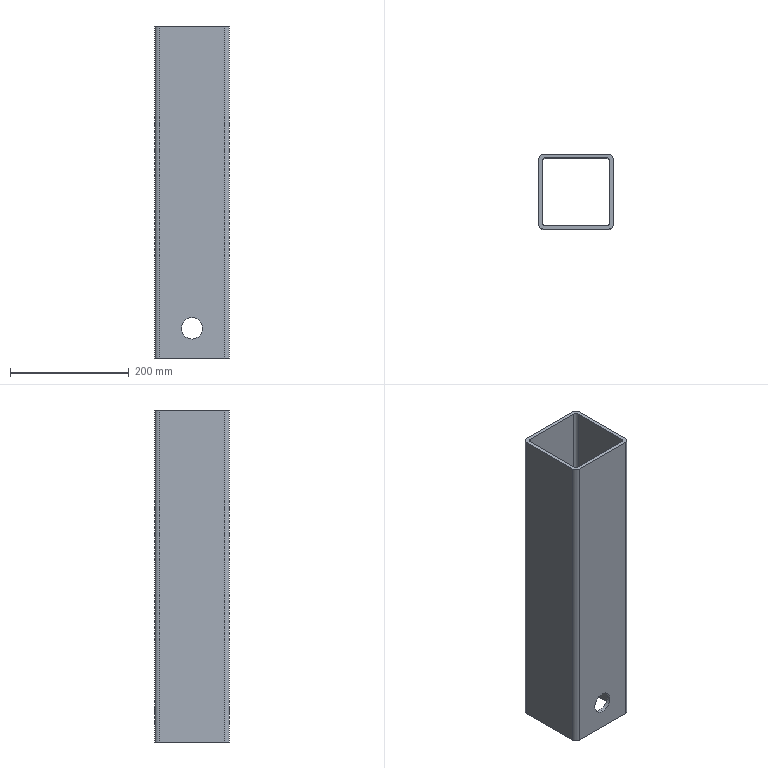Part | SolidWorks | features Fillet 2, Extrusion 1, ICE 1 | 1 solid | 22 faces | box 126 x 126 x 560 mm | volume 1581838 mm3 | cylinder 12 | plane 10 | commonest cylinder face diameters 10 x4 16 x4 36 x4
STEP:
#1=CARTESIAN_POINT('',(63.,6.,32.));
#2=VERTEX_POINT('',#1);
#3=CARTESIAN_POINT('',(63.,6.,68.));
#4=VERTEX_POINT('',#3);
#5=CARTESIAN_POINT('',(63.,6.,50.));
#6=DIRECTION('',(0.,1.,0.));
#7=DIRECTION('',(-1.,0.,0.));
#8=AXIS2_PLACEMENT_3D('',#5,#6,#7);
#9=CIRCLE('',#8,18.);
#10=EDGE_CURVE('',#2,#4,#9,.T.);
#11=ORIENTED_EDGE('',*,*,#10,.T.);
#12=CARTESIAN_POINT('',(63.,0.,68.));
#13=VERTEX_POINT('',#12);
#14=CARTESIAN_POINT('',(63.,260.,68.));
#15=DIRECTION('',(0.,-1.,0.));
#16=VECTOR('',#15,1000.);
#17=LINE('',#14,#16);
#18=EDGE_CURVE('',#4,#13,#17,.T.);
#19=ORIENTED_EDGE('',*,*,#18,.T.);
#20=CARTESIAN_POINT('',(63.,0.,32.));
#21=VERTEX_POINT('',#20);
#22=CARTESIAN_POINT('',(63.,0.,50.));
#23=DIRECTION('',(0.,-1.,0.));
#24=DIRECTION('',(0.,0.,-1.));
#25=AXIS2_PLACEMENT_3D('',#22,#23,#24);
#26=CIRCLE('',#25,18.);
#27=EDGE_CURVE('',#13,#21,#26,.T.);
#28=ORIENTED_EDGE('',*,*,#27,.T.);
#29=CARTESIAN_POINT('',(63.,260.,32.));
#30=DIRECTION('',(0.,-1.,0.));
#31=VECTOR('',#30,1000.);
#32=LINE('',#29,#31);
#33=EDGE_CURVE('',#2,#21,#32,.T.);
#34=ORIENTED_EDGE('',*,*,#33,.F.);
#35=EDGE_LOOP('',(#11,#19,#28,#34));
#36=FACE_OUTER_BOUND('',#35,.T.);
#37=CARTESIAN_POINT('',(63.,260.,50.));
#38=DIRECTION('',(0.,-1.,0.));
#39=DIRECTION('',(0.,0.,-1.));
#40=AXIS2_PLACEMENT_3D('',#37,#38,#39);
#41=CYLINDRICAL_SURFACE('',#40,18.);
#42=ADVANCED_FACE('',(#36),#41,.F.);
#43=CARTESIAN_POINT('',(63.,126.,68.));
#44=VERTEX_POINT('',#43);
#45=CARTESIAN_POINT('',(63.,126.,32.));
#46=VERTEX_POINT('',#45);
#47=CARTESIAN_POINT('',(63.,126.,50.));
#48=DIRECTION('',(0.,-1.,0.));
#49=DIRECTION('',(0.,0.,-1.));
#50=AXIS2_PLACEMENT_3D('',#47,#48,#49);
#51=CIRCLE('',#50,18.);
#52=EDGE_CURVE('',#44,#46,#51,.T.);
#53=ORIENTED_EDGE('',*,*,#52,.F.);
#54=CARTESIAN_POINT('',(63.,120.,68.));
#55=VERTEX_POINT('',#54);
#56=CARTESIAN_POINT('',(63.,260.,68.));
#57=DIRECTION('',(0.,-1.,0.));
#58=VECTOR('',#57,1000.);
#59=LINE('',#56,#58);
#60=EDGE_CURVE('',#44,#55,#59,.T.);
#61=ORIENTED_EDGE('',*,*,#60,.T.);
#62=CARTESIAN_POINT('',(63.,120.,32.));
#63=VERTEX_POINT('',#62);
#64=CARTESIAN_POINT('',(63.,120.,50.));
#65=DIRECTION('',(0.,-1.,0.));
#66=DIRECTION('',(0.,0.,-1.));
#67=AXIS2_PLACEMENT_3D('',#64,#65,#66);
#68=CIRCLE('',#67,18.);
#69=EDGE_CURVE('',#55,#63,#68,.T.);
#70=ORIENTED_EDGE('',*,*,#69,.T.);
#71=CARTESIAN_POINT('',(63.,260.,32.));
#72=DIRECTION('',(0.,-1.,0.));
#73=VECTOR('',#72,1000.);
#74=LINE('',#71,#73);
#75=EDGE_CURVE('',#46,#63,#74,.T.);
#76=ORIENTED_EDGE('',*,*,#75,.F.);
#77=EDGE_LOOP('',(#53,#61,#70,#76));
#78=FACE_OUTER_BOUND('',#77,.T.);
#79=CARTESIAN_POINT('',(63.,260.,50.));
#80=DIRECTION('',(0.,-1.,0.));
#81=DIRECTION('',(0.,0.,-1.));
#82=AXIS2_PLACEMENT_3D('',#79,#80,#81);
#83=CYLINDRICAL_SURFACE('',#82,18.);
#84=ADVANCED_FACE('',(#78),#83,.F.);
#85=CARTESIAN_POINT('',(8.,0.,560.));
#86=VERTEX_POINT('',#85);
#87=CARTESIAN_POINT('',(118.,0.,560.));
#88=VERTEX_POINT('',#87);
#89=CARTESIAN_POINT('',(0.,0.,560.));
#90=DIRECTION('',(1.,0.,0.));
#91=VECTOR('',#90,1000.);
#92=LINE('',#89,#91);
#93=EDGE_CURVE('',#86,#88,#92,.T.);
#94=ORIENTED_EDGE('',*,*,#93,.T.);
#95=CARTESIAN_POINT('',(126.,8.,560.));
#96=VERTEX_POINT('',#95);
#97=CARTESIAN_POINT('',(118.,8.,560.));
#98=DIRECTION('',(0.,0.,1.));
#99=DIRECTION('',(-1.,0.,0.));
#100=AXIS2_PLACEMENT_3D('',#97,#98,#99);
#101=CIRCLE('',#100,8.);
#102=EDGE_CURVE('',#88,#96,#101,.T.);
#103=ORIENTED_EDGE('',*,*,#102,.T.);
#104=CARTESIAN_POINT('',(126.,118.,560.));
#105=VERTEX_POINT('',#104);
#106=CARTESIAN_POINT('',(126.,0.,560.));
#107=DIRECTION('',(0.,1.,0.));
#108=VECTOR('',#107,1000.);
#109=LINE('',#106,#108);
#110=EDGE_CURVE('',#96,#105,#109,.T.);
#111=ORIENTED_EDGE('',*,*,#110,.T.);
#112=CARTESIAN_POINT('',(118.,126.,560.));
#113=VERTEX_POINT('',#112);
#114=CARTESIAN_POINT('',(118.,118.,560.));
#115=DIRECTION('',(0.,0.,1.));
#116=DIRECTION('',(-1.,0.,0.));
#117=AXIS2_PLACEMENT_3D('',#114,#115,#116);
#118=CIRCLE('',#117,8.);
#119=EDGE_CURVE('',#105,#113,#118,.T.);
#120=ORIENTED_EDGE('',*,*,#119,.T.);
#121=CARTESIAN_POINT('',(8.,126.,560.));
#122=VERTEX_POINT('',#121);
#123=CARTESIAN_POINT('',(0.,126.,560.));
#124=DIRECTION('',(-1.,0.,0.));
#125=VECTOR('',#124,1000.);
#126=LINE('',#123,#125);
#127=EDGE_CURVE('',#113,#122,#126,.T.);
#128=ORIENTED_EDGE('',*,*,#127,.T.);
#129=CARTESIAN_POINT('',(0.,118.,560.));
#130=VERTEX_POINT('',#129);
#131=CARTESIAN_POINT('',(8.,118.,560.));
#132=DIRECTION('',(0.,0.,1.));
#133=DIRECTION('',(-1.,0.,0.));
#134=AXIS2_PLACEMENT_3D('',#131,#132,#133);
#135=CIRCLE('',#134,8.);
#136=EDGE_CURVE('',#122,#130,#135,.T.);
#137=ORIENTED_EDGE('',*,*,#136,.T.);
#138=CARTESIAN_POINT('',(0.,8.,560.));
#139=VERTEX_POINT('',#138);
#140=CARTESIAN_POINT('',(0.,0.,560.));
#141=DIRECTION('',(0.,-1.,0.));
#142=VECTOR('',#141,1000.);
#143=LINE('',#140,#142);
#144=EDGE_CURVE('',#130,#139,#143,.T.);
#145=ORIENTED_EDGE('',*,*,#144,.T.);
#146=CARTESIAN_POINT('',(8.,8.,560.));
#147=DIRECTION('',(0.,0.,1.));
#148=DIRECTION('',(-1.,0.,0.));
#149=AXIS2_PLACEMENT_3D('',#146,#147,#148);
#150=CIRCLE('',#149,8.);
#151=EDGE_CURVE('',#139,#86,#150,.T.);
#152=ORIENTED_EDGE('',*,*,#151,.T.);
#153=EDGE_LOOP('',(#94,#103,#111,#120,#128,#137,#145,#152));
#154=FACE_OUTER_BOUND('',#153,.T.);
#155=CARTESIAN_POINT('',(6.,115.,560.));
#156=VERTEX_POINT('',#155);
#157=CARTESIAN_POINT('',(6.,11.,560.));
#158=VERTEX_POINT('',#157);
#159=CARTESIAN_POINT('',(6.,120.,560.));
#160=DIRECTION('',(0.,-1.,0.));
#161=VECTOR('',#160,1000.);
#162=LINE('',#159,#161);
#163=EDGE_CURVE('',#156,#158,#162,.T.);
#164=ORIENTED_EDGE('',*,*,#163,.F.);
#165=CARTESIAN_POINT('',(11.,120.,560.));
#166=VERTEX_POINT('',#165);
#167=CARTESIAN_POINT('',(11.,115.,560.));
#168=DIRECTION('',(0.,0.,-1.));
#169=DIRECTION('',(-1.,0.,0.));
#170=AXIS2_PLACEMENT_3D('',#167,#168,#169);
#171=CIRCLE('',#170,5.);
#172=EDGE_CURVE('',#156,#166,#171,.T.);
#173=ORIENTED_EDGE('',*,*,#172,.T.);
#174=CARTESIAN_POINT('',(115.,120.,560.));
#175=VERTEX_POINT('',#174);
#176=CARTESIAN_POINT('',(6.,120.,560.));
#177=DIRECTION('',(-1.,0.,0.));
#178=VECTOR('',#177,1000.);
#179=LINE('',#176,#178);
#180=EDGE_CURVE('',#175,#166,#179,.T.);
#181=ORIENTED_EDGE('',*,*,#180,.F.);
#182=CARTESIAN_POINT('',(120.,115.,560.));
#183=VERTEX_POINT('',#182);
#184=CARTESIAN_POINT('',(115.,115.,560.));
#185=DIRECTION('',(0.,0.,-1.));
#186=DIRECTION('',(-1.,0.,0.));
#187=AXIS2_PLACEMENT_3D('',#184,#185,#186);
#188=CIRCLE('',#187,5.);
#189=EDGE_CURVE('',#175,#183,#188,.T.);
#190=ORIENTED_EDGE('',*,*,#189,.T.);
#191=CARTESIAN_POINT('',(120.,11.,560.));
#192=VERTEX_POINT('',#191);
#193=CARTESIAN_POINT('',(120.,120.,560.));
#194=DIRECTION('',(0.,1.,0.));
#195=VECTOR('',#194,1000.);
#196=LINE('',#193,#195);
#197=EDGE_CURVE('',#192,#183,#196,.T.);
#198=ORIENTED_EDGE('',*,*,#197,.F.);
#199=CARTESIAN_POINT('',(115.,6.,560.));
#200=VERTEX_POINT('',#199);
#201=CARTESIAN_POINT('',(115.,11.,560.));
#202=DIRECTION('',(0.,0.,-1.));
#203=DIRECTION('',(-1.,0.,0.));
#204=AXIS2_PLACEMENT_3D('',#201,#202,#203);
#205=CIRCLE('',#204,5.);
#206=EDGE_CURVE('',#192,#200,#205,.T.);
#207=ORIENTED_EDGE('',*,*,#206,.T.);
#208=CARTESIAN_POINT('',(11.,6.,560.));
#209=VERTEX_POINT('',#208);
#210=CARTESIAN_POINT('',(6.,6.,560.));
#211=DIRECTION('',(1.,0.,0.));
#212=VECTOR('',#211,1000.);
#213=LINE('',#210,#212);
#214=EDGE_CURVE('',#209,#200,#213,.T.);
#215=ORIENTED_EDGE('',*,*,#214,.F.);
#216=CARTESIAN_POINT('',(11.,11.,560.));
#217=DIRECTION('',(0.,0.,-1.));
#218=DIRECTION('',(-1.,0.,0.));
#219=AXIS2_PLACEMENT_3D('',#216,#217,#218);
#220=CIRCLE('',#219,5.);
#221=EDGE_CURVE('',#209,#158,#220,.T.);
#222=ORIENTED_EDGE('',*,*,#221,.T.);
#223=EDGE_LOOP('',(#164,#173,#181,#190,#198,#207,#215,#222));
#224=FACE_BOUND('',#223,.T.);
#225=CARTESIAN_POINT('',(0.,0.,560.));
#226=DIRECTION('',(0.,0.,-1.));
#227=DIRECTION('',(-1.,0.,0.));
#228=AXIS2_PLACEMENT_3D('',#225,#226,#227);
#229=PLANE('',#228);
#230=ADVANCED_FACE('',(#154,#224),#229,.F.);
#231=CARTESIAN_POINT('',(126.,8.,0.));
#232=VERTEX_POINT('',#231);
#233=CARTESIAN_POINT('',(126.,118.,0.));
#234=VERTEX_POINT('',#233);
#235=CARTESIAN_POINT('',(126.,0.,0.));
#236=DIRECTION('',(0.,1.,0.));
#237=VECTOR('',#236,1000.);
#238=LINE('',#235,#237);
#239=EDGE_CURVE('',#232,#234,#238,.T.);
#240=ORIENTED_EDGE('',*,*,#239,.F.);
#241=CARTESIAN_POINT('',(118.,0.,0.));
#242=VERTEX_POINT('',#241);
#243=CARTESIAN_POINT('',(118.,8.,0.));
#244=DIRECTION('',(0.,0.,-1.));
#245=DIRECTION('',(-1.,0.,0.));
#246=AXIS2_PLACEMENT_3D('',#243,#244,#245);
#247=CIRCLE('',#246,8.);
#248=EDGE_CURVE('',#232,#242,#247,.T.);
#249=ORIENTED_EDGE('',*,*,#248,.T.);
#250=CARTESIAN_POINT('',(8.,0.,0.));
#251=VERTEX_POINT('',#250);
#252=CARTESIAN_POINT('',(0.,0.,0.));
#253=DIRECTION('',(1.,0.,0.));
#254=VECTOR('',#253,1000.);
#255=LINE('',#252,#254);
#256=EDGE_CURVE('',#251,#242,#255,.T.);
#257=ORIENTED_EDGE('',*,*,#256,.F.);
#258=CARTESIAN_POINT('',(0.,8.,0.));
#259=VERTEX_POINT('',#258);
#260=CARTESIAN_POINT('',(8.,8.,0.));
#261=DIRECTION('',(0.,0.,-1.));
#262=DIRECTION('',(-1.,0.,0.));
#263=AXIS2_PLACEMENT_3D('',#260,#261,#262);
#264=CIRCLE('',#263,8.);
#265=EDGE_CURVE('',#251,#259,#264,.T.);
#266=ORIENTED_EDGE('',*,*,#265,.T.);
#267=CARTESIAN_POINT('',(0.,118.,0.));
#268=VERTEX_POINT('',#267);
#269=CARTESIAN_POINT('',(0.,0.,0.));
#270=DIRECTION('',(0.,-1.,0.));
#271=VECTOR('',#270,1000.);
#272=LINE('',#269,#271);
#273=EDGE_CURVE('',#268,#259,#272,.T.);
#274=ORIENTED_EDGE('',*,*,#273,.F.);
#275=CARTESIAN_POINT('',(8.,126.,0.));
#276=VERTEX_POINT('',#275);
#277=CARTESIAN_POINT('',(8.,118.,0.));
#278=DIRECTION('',(0.,0.,-1.));
#279=DIRECTION('',(-1.,0.,0.));
#280=AXIS2_PLACEMENT_3D('',#277,#278,#279);
#281=CIRCLE('',#280,8.);
#282=EDGE_CURVE('',#268,#276,#281,.T.);
#283=ORIENTED_EDGE('',*,*,#282,.T.);
#284=CARTESIAN_POINT('',(118.,126.,0.));
#285=VERTEX_POINT('',#284);
#286=CARTESIAN_POINT('',(0.,126.,0.));
#287=DIRECTION('',(-1.,0.,0.));
#288=VECTOR('',#287,1000.);
#289=LINE('',#286,#288);
#290=EDGE_CURVE('',#285,#276,#289,.T.);
#291=ORIENTED_EDGE('',*,*,#290,.F.);
#292=CARTESIAN_POINT('',(118.,118.,0.));
#293=DIRECTION('',(0.,0.,-1.));
#294=DIRECTION('',(-1.,0.,0.));
#295=AXIS2_PLACEMENT_3D('',#292,#293,#294);
#296=CIRCLE('',#295,8.);
#297=EDGE_CURVE('',#285,#234,#296,.T.);
#298=ORIENTED_EDGE('',*,*,#297,.T.);
#299=EDGE_LOOP('',(#240,#249,#257,#266,#274,#283,#291,#298));
#300=FACE_OUTER_BOUND('',#299,.T.);
#301=CARTESIAN_POINT('',(120.,11.,0.));
#302=VERTEX_POINT('',#301);
#303=CARTESIAN_POINT('',(120.,115.,0.));
#304=VERTEX_POINT('',#303);
#305=CARTESIAN_POINT('',(120.,120.,0.));
#306=DIRECTION('',(0.,1.,0.));
#307=VECTOR('',#306,1000.);
#308=LINE('',#305,#307);
#309=EDGE_CURVE('',#302,#304,#308,.T.);
#310=ORIENTED_EDGE('',*,*,#309,.T.);
#311=CARTESIAN_POINT('',(115.,120.,0.));
#312=VERTEX_POINT('',#311);
#313=CARTESIAN_POINT('',(115.,115.,0.));
#314=DIRECTION('',(0.,0.,1.));
#315=DIRECTION('',(-1.,0.,0.));
#316=AXIS2_PLACEMENT_3D('',#313,#314,#315);
#317=CIRCLE('',#316,5.);
#318=EDGE_CURVE('',#304,#312,#317,.T.);
#319=ORIENTED_EDGE('',*,*,#318,.T.);
#320=CARTESIAN_POINT('',(11.,120.,0.));
#321=VERTEX_POINT('',#320);
#322=CARTESIAN_POINT('',(6.,120.,0.));
#323=DIRECTION('',(-1.,0.,0.));
#324=VECTOR('',#323,1000.);
#325=LINE('',#322,#324);
#326=EDGE_CURVE('',#312,#321,#325,.T.);
#327=ORIENTED_EDGE('',*,*,#326,.T.);
#328=CARTESIAN_POINT('',(6.,115.,0.));
#329=VERTEX_POINT('',#328);
#330=CARTESIAN_POINT('',(11.,115.,0.));
#331=DIRECTION('',(0.,0.,1.));
#332=DIRECTION('',(-1.,0.,0.));
#333=AXIS2_PLACEMENT_3D('',#330,#331,#332);
#334=CIRCLE('',#333,5.);
#335=EDGE_CURVE('',#321,#329,#334,.T.);
#336=ORIENTED_EDGE('',*,*,#335,.T.);
#337=CARTESIAN_POINT('',(6.,11.,0.));
#338=VERTEX_POINT('',#337);
#339=CARTESIAN_POINT('',(6.,120.,0.));
#340=DIRECTION('',(0.,-1.,0.));
#341=VECTOR('',#340,1000.);
#342=LINE('',#339,#341);
#343=EDGE_CURVE('',#329,#338,#342,.T.);
#344=ORIENTED_EDGE('',*,*,#343,.T.);
#345=CARTESIAN_POINT('',(11.,6.,0.));
#346=VERTEX_POINT('',#345);
#347=CARTESIAN_POINT('',(11.,11.,0.));
#348=DIRECTION('',(0.,0.,1.));
#349=DIRECTION('',(-1.,0.,0.));
#350=AXIS2_PLACEMENT_3D('',#347,#348,#349);
#351=CIRCLE('',#350,5.);
#352=EDGE_CURVE('',#338,#346,#351,.T.);
#353=ORIENTED_EDGE('',*,*,#352,.T.);
#354=CARTESIAN_POINT('',(115.,6.,0.));
#355=VERTEX_POINT('',#354);
#356=CARTESIAN_POINT('',(6.,6.,0.));
#357=DIRECTION('',(1.,0.,0.));
#358=VECTOR('',#357,1000.);
#359=LINE('',#356,#358);
#360=EDGE_CURVE('',#346,#355,#359,.T.);
#361=ORIENTED_EDGE('',*,*,#360,.T.);
#362=CARTESIAN_POINT('',(115.,11.,0.));
#363=DIRECTION('',(0.,0.,1.));
#364=DIRECTION('',(-1.,0.,0.));
#365=AXIS2_PLACEMENT_3D('',#362,#363,#364);
#366=CIRCLE('',#365,5.);
#367=EDGE_CURVE('',#355,#302,#366,.T.);
#368=ORIENTED_EDGE('',*,*,#367,.T.);
#369=EDGE_LOOP('',(#310,#319,#327,#336,#344,#353,#361,#368));
#370=FACE_BOUND('',#369,.T.);
#371=CARTESIAN_POINT('',(0.,0.,0.));
#372=DIRECTION('',(0.,0.,-1.));
#373=DIRECTION('',(-1.,0.,0.));
#374=AXIS2_PLACEMENT_3D('',#371,#372,#373);
#375=PLANE('',#374);
#376=ADVANCED_FACE('',(#300,#370),#375,.T.);
#377=ORIENTED_EDGE('',*,*,#273,.T.);
#378=CARTESIAN_POINT('',(0.,8.,560.));
#379=DIRECTION('',(0.,0.,1.));
#380=VECTOR('',#379,1000.);
#381=LINE('',#378,#380);
#382=EDGE_CURVE('',#259,#139,#381,.T.);
#383=ORIENTED_EDGE('',*,*,#382,.T.);
#384=ORIENTED_EDGE('',*,*,#144,.F.);
#385=CARTESIAN_POINT('',(0.,118.,560.));
#386=DIRECTION('',(0.,0.,-1.));
#387=VECTOR('',#386,1000.);
#388=LINE('',#385,#387);
#389=EDGE_CURVE('',#130,#268,#388,.T.);
#390=ORIENTED_EDGE('',*,*,#389,.T.);
#391=EDGE_LOOP('',(#377,#383,#384,#390));
#392=FACE_OUTER_BOUND('',#391,.T.);
#393=CARTESIAN_POINT('',(0.,0.,560.));
#394=DIRECTION('',(1.,0.,0.));
#395=DIRECTION('',(0.,0.,-1.));
#396=AXIS2_PLACEMENT_3D('',#393,#394,#395);
#397=PLANE('',#396);
#398=ADVANCED_FACE('',(#392),#397,.F.);
#399=CARTESIAN_POINT('',(63.,0.,50.));
#400=DIRECTION('',(0.,-1.,0.));
#401=DIRECTION('',(0.,0.,-1.));
#402=AXIS2_PLACEMENT_3D('',#399,#400,#401);
#403=CIRCLE('',#402,18.);
#404=EDGE_CURVE('',#21,#13,#403,.T.);
#405=ORIENTED_EDGE('',*,*,#404,.F.);
#406=ORIENTED_EDGE('',*,*,#27,.F.);
#407=EDGE_LOOP('',(#405,#406));
#408=FACE_BOUND('',#407,.T.);
#409=ORIENTED_EDGE('',*,*,#256,.T.);
#410=CARTESIAN_POINT('',(118.,0.,560.));
#411=DIRECTION('',(0.,0.,1.));
#412=VECTOR('',#411,1000.);
#413=LINE('',#410,#412);
#414=EDGE_CURVE('',#242,#88,#413,.T.);
#415=ORIENTED_EDGE('',*,*,#414,.T.);
#416=ORIENTED_EDGE('',*,*,#93,.F.);
#417=CARTESIAN_POINT('',(8.,0.,560.));
#418=DIRECTION('',(0.,0.,-1.));
#419=VECTOR('',#418,1000.);
#420=LINE('',#417,#419);
#421=EDGE_CURVE('',#86,#251,#420,.T.);
#422=ORIENTED_EDGE('',*,*,#421,.T.);
#423=EDGE_LOOP('',(#409,#415,#416,#422));
#424=FACE_OUTER_BOUND('',#423,.T.);
#425=CARTESIAN_POINT('',(0.,0.,560.));
#426=DIRECTION('',(0.,1.,0.));
#427=DIRECTION('',(0.,0.,1.));
#428=AXIS2_PLACEMENT_3D('',#425,#426,#427);
#429=PLANE('',#428);
#430=ADVANCED_FACE('',(#408,#424),#429,.F.);
#431=ORIENTED_EDGE('',*,*,#110,.F.);
#432=CARTESIAN_POINT('',(126.,8.,560.));
#433=DIRECTION('',(0.,0.,-1.));
#434=VECTOR('',#433,1000.);
#435=LINE('',#432,#434);
#436=EDGE_CURVE('',#96,#232,#435,.T.);
#437=ORIENTED_EDGE('',*,*,#436,.T.);
#438=ORIENTED_EDGE('',*,*,#239,.T.);
#439=CARTESIAN_POINT('',(126.,118.,560.));
#440=DIRECTION('',(0.,0.,1.));
#441=VECTOR('',#440,1000.);
#442=LINE('',#439,#441);
#443=EDGE_CURVE('',#234,#105,#442,.T.);
#444=ORIENTED_EDGE('',*,*,#443,.T.);
#445=EDGE_LOOP('',(#431,#437,#438,#444));
#446=FACE_OUTER_BOUND('',#445,.T.);
#447=CARTESIAN_POINT('',(126.,0.,560.));
#448=DIRECTION('',(-1.,0.,0.));
#449=DIRECTION('',(0.,0.,1.));
#450=AXIS2_PLACEMENT_3D('',#447,#448,#449);
#451=PLANE('',#450);
#452=ADVANCED_FACE('',(#446),#451,.F.);
#453=CARTESIAN_POINT('',(63.,126.,50.));
#454=DIRECTION('',(0.,-1.,0.));
#455=DIRECTION('',(0.,0.,-1.));
#456=AXIS2_PLACEMENT_3D('',#453,#454,#455);
#457=CIRCLE('',#456,18.);
#458=EDGE_CURVE('',#46,#44,#457,.T.);
#459=ORIENTED_EDGE('',*,*,#458,.T.);
#460=ORIENTED_EDGE('',*,*,#52,.T.);
#461=EDGE_LOOP('',(#459,#460));
#462=FACE_BOUND('',#461,.T.);
#463=ORIENTED_EDGE('',*,*,#290,.T.);
#464=CARTESIAN_POINT('',(8.,126.,560.));
#465=DIRECTION('',(0.,0.,1.));
#466=VECTOR('',#465,1000.);
#467=LINE('',#464,#466);
#468=EDGE_CURVE('',#276,#122,#467,.T.);
#469=ORIENTED_EDGE('',*,*,#468,.T.);
#470=ORIENTED_EDGE('',*,*,#127,.F.);
#471=CARTESIAN_POINT('',(118.,126.,560.));
#472=DIRECTION('',(0.,0.,-1.));
#473=VECTOR('',#472,1000.);
#474=LINE('',#471,#473);
#475=EDGE_CURVE('',#113,#285,#474,.T.);
#476=ORIENTED_EDGE('',*,*,#475,.T.);
#477=EDGE_LOOP('',(#463,#469,#470,#476));
#478=FACE_OUTER_BOUND('',#477,.T.);
#479=CARTESIAN_POINT('',(0.,126.,560.));
#480=DIRECTION('',(0.,-1.,0.));
#481=DIRECTION('',(0.,0.,-1.));
#482=AXIS2_PLACEMENT_3D('',#479,#480,#481);
#483=PLANE('',#482);
#484=ADVANCED_FACE('',(#462,#478),#483,.F.);
#485=ORIENTED_EDGE('',*,*,#163,.T.);
#486=CARTESIAN_POINT('',(6.,11.,0.));
#487=DIRECTION('',(0.,0.,-1.));
#488=VECTOR('',#487,1000.);
#489=LINE('',#486,#488);
#490=EDGE_CURVE('',#158,#338,#489,.T.);
#491=ORIENTED_EDGE('',*,*,#490,.T.);
#492=ORIENTED_EDGE('',*,*,#343,.F.);
#493=CARTESIAN_POINT('',(6.,115.,560.));
#494=DIRECTION('',(0.,0.,1.));
#495=VECTOR('',#494,1000.);
#496=LINE('',#493,#495);
#497=EDGE_CURVE('',#329,#156,#496,.T.);
#498=ORIENTED_EDGE('',*,*,#497,.T.);
#499=EDGE_LOOP('',(#485,#491,#492,#498));
#500=FACE_OUTER_BOUND('',#499,.T.);
#501=CARTESIAN_POINT('',(6.,120.,560.));
#502=DIRECTION('',(1.,0.,0.));
#503=DIRECTION('',(0.,1.,0.));
#504=AXIS2_PLACEMENT_3D('',#501,#502,#503);
#505=PLANE('',#504);
#506=ADVANCED_FACE('',(#500),#505,.T.);
#507=ORIENTED_EDGE('',*,*,#10,.F.);
#508=CARTESIAN_POINT('',(63.,6.,50.));
#509=DIRECTION('',(0.,1.,0.));
#510=DIRECTION('',(-1.,0.,0.));
#511=AXIS2_PLACEMENT_3D('',#508,#509,#510);
#512=CIRCLE('',#511,18.);
#513=EDGE_CURVE('',#4,#2,#512,.T.);
#514=ORIENTED_EDGE('',*,*,#513,.F.);
#515=EDGE_LOOP('',(#507,#514));
#516=FACE_BOUND('',#515,.T.);
#517=ORIENTED_EDGE('',*,*,#360,.F.);
#518=CARTESIAN_POINT('',(11.,6.,560.));
#519=DIRECTION('',(0.,0.,1.));
#520=VECTOR('',#519,1000.);
#521=LINE('',#518,#520);
#522=EDGE_CURVE('',#346,#209,#521,.T.);
#523=ORIENTED_EDGE('',*,*,#522,.T.);
#524=ORIENTED_EDGE('',*,*,#214,.T.);
#525=CARTESIAN_POINT('',(115.,6.,0.));
#526=DIRECTION('',(0.,0.,-1.));
#527=VECTOR('',#526,1000.);
#528=LINE('',#525,#527);
#529=EDGE_CURVE('',#200,#355,#528,.T.);
#530=ORIENTED_EDGE('',*,*,#529,.T.);
#531=EDGE_LOOP('',(#517,#523,#524,#530));
#532=FACE_OUTER_BOUND('',#531,.T.);
#533=CARTESIAN_POINT('',(6.,6.,560.));
#534=DIRECTION('',(0.,1.,0.));
#535=DIRECTION('',(-1.,0.,0.));
#536=AXIS2_PLACEMENT_3D('',#533,#534,#535);
#537=PLANE('',#536);
#538=ADVANCED_FACE('',(#516,#532),#537,.T.);
#539=ORIENTED_EDGE('',*,*,#309,.F.);
#540=CARTESIAN_POINT('',(120.,11.,560.));
#541=DIRECTION('',(0.,0.,1.));
#542=VECTOR('',#541,1000.);
#543=LINE('',#540,#542);
#544=EDGE_CURVE('',#302,#192,#543,.T.);
#545=ORIENTED_EDGE('',*,*,#544,.T.);
#546=ORIENTED_EDGE('',*,*,#197,.T.);
#547=CARTESIAN_POINT('',(120.,115.,0.));
#548=DIRECTION('',(0.,0.,-1.));
#549=VECTOR('',#548,1000.);
#550=LINE('',#547,#549);
#551=EDGE_CURVE('',#183,#304,#550,.T.);
#552=ORIENTED_EDGE('',*,*,#551,.T.);
#553=EDGE_LOOP('',(#539,#545,#546,#552));
#554=FACE_OUTER_BOUND('',#553,.T.);
#555=CARTESIAN_POINT('',(120.,120.,560.));
#556=DIRECTION('',(-1.,0.,0.));
#557=DIRECTION('',(0.,-1.,0.));
#558=AXIS2_PLACEMENT_3D('',#555,#556,#557);
#559=PLANE('',#558);
#560=ADVANCED_FACE('',(#554),#559,.T.);
#561=CARTESIAN_POINT('',(63.,120.,50.));
#562=DIRECTION('',(0.,-1.,0.));
#563=DIRECTION('',(0.,0.,-1.));
#564=AXIS2_PLACEMENT_3D('',#561,#562,#563);
#565=CIRCLE('',#564,18.);
#566=EDGE_CURVE('',#63,#55,#565,.T.);
#567=ORIENTED_EDGE('',*,*,#566,.F.);
#568=ORIENTED_EDGE('',*,*,#69,.F.);
#569=EDGE_LOOP('',(#567,#568));
#570=FACE_BOUND('',#569,.T.);
#571=ORIENTED_EDGE('',*,*,#326,.F.);
#572=CARTESIAN_POINT('',(115.,120.,560.));
#573=DIRECTION('',(0.,0.,1.));
#574=VECTOR('',#573,1000.);
#575=LINE('',#572,#574);
#576=EDGE_CURVE('',#312,#175,#575,.T.);
#577=ORIENTED_EDGE('',*,*,#576,.T.);
#578=ORIENTED_EDGE('',*,*,#180,.T.);
#579=CARTESIAN_POINT('',(11.,120.,0.));
#580=DIRECTION('',(0.,0.,-1.));
#581=VECTOR('',#580,1000.);
#582=LINE('',#579,#581);
#583=EDGE_CURVE('',#166,#321,#582,.T.);
#584=ORIENTED_EDGE('',*,*,#583,.T.);
#585=EDGE_LOOP('',(#571,#577,#578,#584));
#586=FACE_OUTER_BOUND('',#585,.T.);
#587=CARTESIAN_POINT('',(6.,120.,560.));
#588=DIRECTION('',(0.,-1.,0.));
#589=DIRECTION('',(0.,0.,-1.));
#590=AXIS2_PLACEMENT_3D('',#587,#588,#589);
#591=PLANE('',#590);
#592=ADVANCED_FACE('',(#570,#586),#591,.T.);
#593=ORIENTED_EDGE('',*,*,#102,.F.);
#594=ORIENTED_EDGE('',*,*,#414,.F.);
#595=ORIENTED_EDGE('',*,*,#248,.F.);
#596=ORIENTED_EDGE('',*,*,#436,.F.);
#597=EDGE_LOOP('',(#593,#594,#595,#596));
#598=FACE_OUTER_BOUND('',#597,.T.);
#599=CARTESIAN_POINT('',(118.,8.,560.));
#600=DIRECTION('',(0.,0.,-1.));
#601=DIRECTION('',(-1.,0.,0.));
#602=AXIS2_PLACEMENT_3D('',#599,#600,#601);
#603=CYLINDRICAL_SURFACE('',#602,8.);
#604=ADVANCED_FACE('',(#598),#603,.T.);
#605=ORIENTED_EDGE('',*,*,#151,.F.);
#606=ORIENTED_EDGE('',*,*,#382,.F.);
#607=ORIENTED_EDGE('',*,*,#265,.F.);
#608=ORIENTED_EDGE('',*,*,#421,.F.);
#609=EDGE_LOOP('',(#605,#606,#607,#608));
#610=FACE_OUTER_BOUND('',#609,.T.);
#611=CARTESIAN_POINT('',(8.,8.,560.));
#612=DIRECTION('',(0.,0.,-1.));
#613=DIRECTION('',(-1.,0.,0.));
#614=AXIS2_PLACEMENT_3D('',#611,#612,#613);
#615=CYLINDRICAL_SURFACE('',#614,8.);
#616=ADVANCED_FACE('',(#610),#615,.T.);
#617=ORIENTED_EDGE('',*,*,#136,.F.);
#618=ORIENTED_EDGE('',*,*,#468,.F.);
#619=ORIENTED_EDGE('',*,*,#282,.F.);
#620=ORIENTED_EDGE('',*,*,#389,.F.);
#621=EDGE_LOOP('',(#617,#618,#619,#620));
#622=FACE_OUTER_BOUND('',#621,.T.);
#623=CARTESIAN_POINT('',(8.,118.,560.));
#624=DIRECTION('',(0.,0.,-1.));
#625=DIRECTION('',(-1.,0.,0.));
#626=AXIS2_PLACEMENT_3D('',#623,#624,#625);
#627=CYLINDRICAL_SURFACE('',#626,8.);
#628=ADVANCED_FACE('',(#622),#627,.T.);
#629=ORIENTED_EDGE('',*,*,#119,.F.);
#630=ORIENTED_EDGE('',*,*,#443,.F.);
#631=ORIENTED_EDGE('',*,*,#297,.F.);
#632=ORIENTED_EDGE('',*,*,#475,.F.);
#633=EDGE_LOOP('',(#629,#630,#631,#632));
#634=FACE_OUTER_BOUND('',#633,.T.);
#635=CARTESIAN_POINT('',(118.,118.,560.));
#636=DIRECTION('',(0.,0.,-1.));
#637=DIRECTION('',(-1.,0.,0.));
#638=AXIS2_PLACEMENT_3D('',#635,#636,#637);
#639=CYLINDRICAL_SURFACE('',#638,8.);
#640=ADVANCED_FACE('',(#634),#639,.T.);
#641=ORIENTED_EDGE('',*,*,#221,.F.);
#642=ORIENTED_EDGE('',*,*,#522,.F.);
#643=ORIENTED_EDGE('',*,*,#352,.F.);
#644=ORIENTED_EDGE('',*,*,#490,.F.);
#645=EDGE_LOOP('',(#641,#642,#643,#644));
#646=FACE_OUTER_BOUND('',#645,.T.);
#647=CARTESIAN_POINT('',(11.,11.,560.));
#648=DIRECTION('',(0.,0.,1.));
#649=DIRECTION('',(1.,0.,0.));
#650=AXIS2_PLACEMENT_3D('',#647,#648,#649);
#651=CYLINDRICAL_SURFACE('',#650,5.);
#652=ADVANCED_FACE('',(#646),#651,.F.);
#653=ORIENTED_EDGE('',*,*,#206,.F.);
#654=ORIENTED_EDGE('',*,*,#544,.F.);
#655=ORIENTED_EDGE('',*,*,#367,.F.);
#656=ORIENTED_EDGE('',*,*,#529,.F.);
#657=EDGE_LOOP('',(#653,#654,#655,#656));
#658=FACE_OUTER_BOUND('',#657,.T.);
#659=CARTESIAN_POINT('',(115.,11.,560.));
#660=DIRECTION('',(0.,0.,1.));
#661=DIRECTION('',(1.,0.,0.));
#662=AXIS2_PLACEMENT_3D('',#659,#660,#661);
#663=CYLINDRICAL_SURFACE('',#662,5.);
#664=ADVANCED_FACE('',(#658),#663,.F.);
#665=ORIENTED_EDGE('',*,*,#189,.F.);
#666=ORIENTED_EDGE('',*,*,#576,.F.);
#667=ORIENTED_EDGE('',*,*,#318,.F.);
#668=ORIENTED_EDGE('',*,*,#551,.F.);
#669=EDGE_LOOP('',(#665,#666,#667,#668));
#670=FACE_OUTER_BOUND('',#669,.T.);
#671=CARTESIAN_POINT('',(115.,115.,560.));
#672=DIRECTION('',(0.,0.,1.));
#673=DIRECTION('',(1.,0.,0.));
#674=AXIS2_PLACEMENT_3D('',#671,#672,#673);
#675=CYLINDRICAL_SURFACE('',#674,5.);
#676=ADVANCED_FACE('',(#670),#675,.F.);
#677=ORIENTED_EDGE('',*,*,#172,.F.);
#678=ORIENTED_EDGE('',*,*,#497,.F.);
#679=ORIENTED_EDGE('',*,*,#335,.F.);
#680=ORIENTED_EDGE('',*,*,#583,.F.);
#681=EDGE_LOOP('',(#677,#678,#679,#680));
#682=FACE_OUTER_BOUND('',#681,.T.);
#683=CARTESIAN_POINT('',(11.,115.,560.));
#684=DIRECTION('',(0.,0.,1.));
#685=DIRECTION('',(1.,0.,0.));
#686=AXIS2_PLACEMENT_3D('',#683,#684,#685);
#687=CYLINDRICAL_SURFACE('',#686,5.);
#688=ADVANCED_FACE('',(#682),#687,.F.);
#689=ORIENTED_EDGE('',*,*,#60,.F.);
#690=ORIENTED_EDGE('',*,*,#458,.F.);
#691=ORIENTED_EDGE('',*,*,#75,.T.);
#692=ORIENTED_EDGE('',*,*,#566,.T.);
#693=EDGE_LOOP('',(#689,#690,#691,#692));
#694=FACE_OUTER_BOUND('',#693,.T.);
#695=CARTESIAN_POINT('',(63.,260.,50.));
#696=DIRECTION('',(0.,-1.,0.));
#697=DIRECTION('',(0.,0.,-1.));
#698=AXIS2_PLACEMENT_3D('',#695,#696,#697);
#699=CYLINDRICAL_SURFACE('',#698,18.);
#700=ADVANCED_FACE('',(#694),#699,.F.);
#701=ORIENTED_EDGE('',*,*,#18,.F.);
#702=ORIENTED_EDGE('',*,*,#513,.T.);
#703=ORIENTED_EDGE('',*,*,#33,.T.);
#704=ORIENTED_EDGE('',*,*,#404,.T.);
#705=EDGE_LOOP('',(#701,#702,#703,#704));
#706=FACE_OUTER_BOUND('',#705,.T.);
#707=CARTESIAN_POINT('',(63.,260.,50.));
#708=DIRECTION('',(0.,-1.,0.));
#709=DIRECTION('',(0.,0.,-1.));
#710=AXIS2_PLACEMENT_3D('',#707,#708,#709);
#711=CYLINDRICAL_SURFACE('',#710,18.);
#712=ADVANCED_FACE('',(#706),#711,.F.);
#713=CLOSED_SHELL('',(#42,#84,#230,#376,#398,#430,#452,#484,#506,#538,#560,#592,#604,#616,#628,#640,#652,#664,#676,#688,#700,#712));
#714=MANIFOLD_SOLID_BREP('',#713);
#715=CARTESIAN_POINT('',(0.,0.,0.));
#716=DIRECTION('',(0.,0.,1.));
#717=DIRECTION('',(1.,0.,0.));
#718=AXIS2_PLACEMENT_3D('',#715,#716,#717);
#719=(LENGTH_UNIT()NAMED_UNIT(*)SI_UNIT(.MILLI.,.METRE.));
#720=UNCERTAINTY_MEASURE_WITH_UNIT(LENGTH_MEASURE(0.00001),#719,'','');
#721=(NAMED_UNIT(*)PLANE_ANGLE_UNIT()SI_UNIT($,.RADIAN.));
#722=(NAMED_UNIT(*)SI_UNIT($,.STERADIAN.)SOLID_ANGLE_UNIT());
#723=(GEOMETRIC_REPRESENTATION_CONTEXT(3)GLOBAL_UNCERTAINTY_ASSIGNED_CONTEXT((#720))GLOBAL_UNIT_ASSIGNED_CONTEXT((#719,#721,#722))REPRESENTATION_CONTEXT('',''));
#724=ADVANCED_BREP_SHAPE_REPRESENTATION('',(#714,#718),#723);